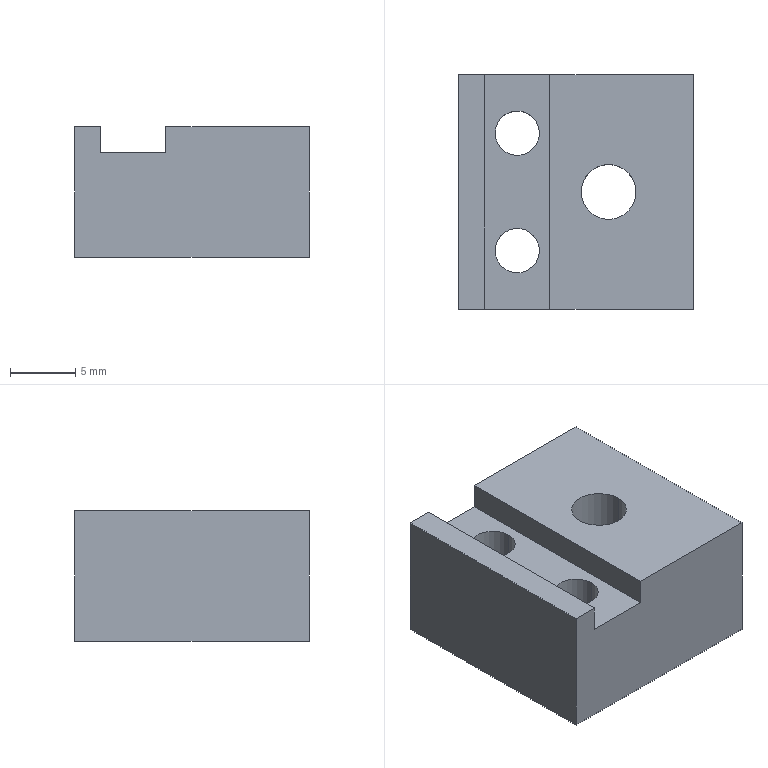Part | STEP file | B10 | 1 solid | 22 faces | box 18 x 18 x 10 mm | volume 2612 mm3 | plane 12 | cylinder 10 | commonest cylinder face diameters 3.4 x4 6.5 x4 4.2 x2